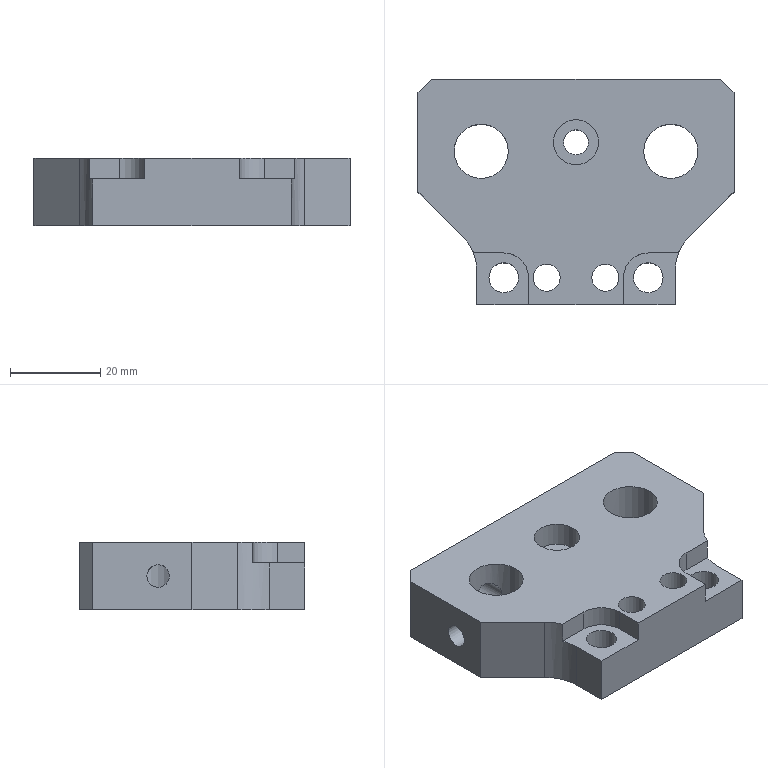Part | NX | features BREP 1 | 1 solid | 34 faces | box 70 x 50 x 15 mm | volume 37859 mm3 | plane 19 | cylinder 15 | commonest cylinder face diameters 5 x3 6 x2 6.6 x2 11 x2 12 x2 20 x2
STEP:
#1=CARTESIAN_POINT('',(35.,22.,0.));
#2=VERTEX_POINT('',#1);
#3=CARTESIAN_POINT('',(32.,25.,0.));
#4=VERTEX_POINT('',#3);
#5=CARTESIAN_POINT('',(35.,22.,0.));
#6=DIRECTION('',(-0.7071,0.7071,0.));
#7=VECTOR('',#6,1000.);
#8=LINE('',#5,#7);
#9=EDGE_CURVE('',#2,#4,#8,.T.);
#10=ORIENTED_EDGE('',*,*,#9,.F.);
#11=CARTESIAN_POINT('',(35.,0.,0.));
#12=VERTEX_POINT('',#11);
#13=CARTESIAN_POINT('',(35.,0.,0.));
#14=DIRECTION('',(0.,1.,0.));
#15=VECTOR('',#14,1000.);
#16=LINE('',#13,#15);
#17=EDGE_CURVE('',#12,#2,#16,.T.);
#18=ORIENTED_EDGE('',*,*,#17,.F.);
#19=CARTESIAN_POINT('',(24.929,-10.071,0.));
#20=VERTEX_POINT('',#19);
#21=CARTESIAN_POINT('',(24.929,-10.071,0.));
#22=DIRECTION('',(0.7071,0.7071,0.));
#23=VECTOR('',#22,1000.);
#24=LINE('',#21,#23);
#25=EDGE_CURVE('',#20,#12,#24,.T.);
#26=ORIENTED_EDGE('',*,*,#25,.F.);
#27=CARTESIAN_POINT('',(22.,-17.142,0.));
#28=VERTEX_POINT('',#27);
#29=CARTESIAN_POINT('',(32.,-17.142,0.));
#30=DIRECTION('',(0.,0.,-1.));
#31=DIRECTION('',(1.,0.,0.));
#32=AXIS2_PLACEMENT_3D('',#29,#30,#31);
#33=CIRCLE('',#32,10.);
#34=EDGE_CURVE('',#28,#20,#33,.T.);
#35=ORIENTED_EDGE('',*,*,#34,.F.);
#36=CARTESIAN_POINT('',(22.,-25.,0.));
#37=VERTEX_POINT('',#36);
#38=CARTESIAN_POINT('',(22.,0.,0.));
#39=DIRECTION('',(0.,1.,0.));
#40=VECTOR('',#39,1000.);
#41=LINE('',#38,#40);
#42=EDGE_CURVE('',#37,#28,#41,.T.);
#43=ORIENTED_EDGE('',*,*,#42,.F.);
#44=CARTESIAN_POINT('',(-22.,-25.,0.));
#45=VERTEX_POINT('',#44);
#46=CARTESIAN_POINT('',(0.,-25.,0.));
#47=DIRECTION('',(1.,0.,0.));
#48=VECTOR('',#47,1000.);
#49=LINE('',#46,#48);
#50=EDGE_CURVE('',#45,#37,#49,.T.);
#51=ORIENTED_EDGE('',*,*,#50,.F.);
#52=CARTESIAN_POINT('',(-22.,-17.142,0.));
#53=VERTEX_POINT('',#52);
#54=CARTESIAN_POINT('',(-22.,0.,0.));
#55=DIRECTION('',(0.,-1.,0.));
#56=VECTOR('',#55,1000.);
#57=LINE('',#54,#56);
#58=EDGE_CURVE('',#53,#45,#57,.T.);
#59=ORIENTED_EDGE('',*,*,#58,.F.);
#60=CARTESIAN_POINT('',(-24.929,-10.071,0.));
#61=VERTEX_POINT('',#60);
#62=CARTESIAN_POINT('',(-32.,-17.142,0.));
#63=DIRECTION('',(0.,0.,-1.));
#64=DIRECTION('',(1.,0.,0.));
#65=AXIS2_PLACEMENT_3D('',#62,#63,#64);
#66=CIRCLE('',#65,10.);
#67=EDGE_CURVE('',#61,#53,#66,.T.);
#68=ORIENTED_EDGE('',*,*,#67,.F.);
#69=CARTESIAN_POINT('',(-35.,0.,0.));
#70=VERTEX_POINT('',#69);
#71=CARTESIAN_POINT('',(-35.,0.,0.));
#72=DIRECTION('',(0.7071,-0.7071,0.));
#73=VECTOR('',#72,1000.);
#74=LINE('',#71,#73);
#75=EDGE_CURVE('',#70,#61,#74,.T.);
#76=ORIENTED_EDGE('',*,*,#75,.F.);
#77=CARTESIAN_POINT('',(-35.,22.,0.));
#78=VERTEX_POINT('',#77);
#79=CARTESIAN_POINT('',(-35.,0.,0.));
#80=DIRECTION('',(0.,-1.,0.));
#81=VECTOR('',#80,1000.);
#82=LINE('',#79,#81);
#83=EDGE_CURVE('',#78,#70,#82,.T.);
#84=ORIENTED_EDGE('',*,*,#83,.F.);
#85=CARTESIAN_POINT('',(-32.,25.,0.));
#86=VERTEX_POINT('',#85);
#87=CARTESIAN_POINT('',(-32.,25.,0.));
#88=DIRECTION('',(-0.7071,-0.7071,0.));
#89=VECTOR('',#88,1000.);
#90=LINE('',#87,#89);
#91=EDGE_CURVE('',#86,#78,#90,.T.);
#92=ORIENTED_EDGE('',*,*,#91,.F.);
#93=CARTESIAN_POINT('',(0.,25.,0.));
#94=DIRECTION('',(-1.,0.,0.));
#95=VECTOR('',#94,1000.);
#96=LINE('',#93,#95);
#97=EDGE_CURVE('',#4,#86,#96,.T.);
#98=ORIENTED_EDGE('',*,*,#97,.F.);
#99=EDGE_LOOP('',(#10,#18,#26,#35,#43,#51,#59,#68,#76,#84,#92,#98));
#100=FACE_BOUND('',#99,.T.);
#101=CARTESIAN_POINT('',(-27.,9.,0.));
#102=VERTEX_POINT('',#101);
#103=CARTESIAN_POINT('',(-21.,9.,0.));
#104=DIRECTION('',(0.,0.,-1.));
#105=DIRECTION('',(-1.,0.,0.));
#106=AXIS2_PLACEMENT_3D('',#103,#104,#105);
#107=CIRCLE('',#106,6.);
#108=EDGE_CURVE('',#102,#102,#107,.T.);
#109=ORIENTED_EDGE('',*,*,#108,.F.);
#110=EDGE_LOOP('',(#109));
#111=FACE_BOUND('',#110,.T.);
#112=CARTESIAN_POINT('',(15.,9.,0.));
#113=VERTEX_POINT('',#112);
#114=CARTESIAN_POINT('',(21.,9.,0.));
#115=DIRECTION('',(0.,0.,-1.));
#116=DIRECTION('',(-1.,0.,0.));
#117=AXIS2_PLACEMENT_3D('',#114,#115,#116);
#118=CIRCLE('',#117,6.);
#119=EDGE_CURVE('',#113,#113,#118,.T.);
#120=ORIENTED_EDGE('',*,*,#119,.F.);
#121=EDGE_LOOP('',(#120));
#122=FACE_BOUND('',#121,.T.);
#123=CARTESIAN_POINT('',(2.75,11.,0.));
#124=VERTEX_POINT('',#123);
#125=CARTESIAN_POINT('',(0.,11.,0.));
#126=DIRECTION('',(0.,0.,-1.));
#127=DIRECTION('',(1.,0.,0.));
#128=AXIS2_PLACEMENT_3D('',#125,#126,#127);
#129=CIRCLE('',#128,2.75);
#130=EDGE_CURVE('',#124,#124,#129,.T.);
#131=ORIENTED_EDGE('',*,*,#130,.F.);
#132=EDGE_LOOP('',(#131));
#133=FACE_BOUND('',#132,.T.);
#134=CARTESIAN_POINT('',(9.5,-19.,0.));
#135=VERTEX_POINT('',#134);
#136=CARTESIAN_POINT('',(6.5,-19.,0.));
#137=DIRECTION('',(0.,0.,-1.));
#138=DIRECTION('',(1.,0.,0.));
#139=AXIS2_PLACEMENT_3D('',#136,#137,#138);
#140=CIRCLE('',#139,3.);
#141=EDGE_CURVE('',#135,#135,#140,.T.);
#142=ORIENTED_EDGE('',*,*,#141,.F.);
#143=EDGE_LOOP('',(#142));
#144=FACE_BOUND('',#143,.T.);
#145=CARTESIAN_POINT('',(-3.5,-19.,0.));
#146=VERTEX_POINT('',#145);
#147=CARTESIAN_POINT('',(-6.5,-19.,0.));
#148=DIRECTION('',(0.,0.,-1.));
#149=DIRECTION('',(1.,0.,0.));
#150=AXIS2_PLACEMENT_3D('',#147,#148,#149);
#151=CIRCLE('',#150,3.);
#152=EDGE_CURVE('',#146,#146,#151,.T.);
#153=ORIENTED_EDGE('',*,*,#152,.F.);
#154=EDGE_LOOP('',(#153));
#155=FACE_BOUND('',#154,.T.);
#156=CARTESIAN_POINT('',(-12.7,-19.,0.));
#157=VERTEX_POINT('',#156);
#158=CARTESIAN_POINT('',(-16.,-19.,0.));
#159=DIRECTION('',(0.,0.,-1.));
#160=DIRECTION('',(1.,0.,0.));
#161=AXIS2_PLACEMENT_3D('',#158,#159,#160);
#162=CIRCLE('',#161,3.3);
#163=EDGE_CURVE('',#157,#157,#162,.T.);
#164=ORIENTED_EDGE('',*,*,#163,.F.);
#165=EDGE_LOOP('',(#164));
#166=FACE_BOUND('',#165,.T.);
#167=CARTESIAN_POINT('',(19.3,-19.,0.));
#168=VERTEX_POINT('',#167);
#169=CARTESIAN_POINT('',(16.,-19.,0.));
#170=DIRECTION('',(0.,0.,-1.));
#171=DIRECTION('',(1.,0.,0.));
#172=AXIS2_PLACEMENT_3D('',#169,#170,#171);
#173=CIRCLE('',#172,3.3);
#174=EDGE_CURVE('',#168,#168,#173,.T.);
#175=ORIENTED_EDGE('',*,*,#174,.F.);
#176=EDGE_LOOP('',(#175));
#177=FACE_BOUND('',#176,.T.);
#178=CARTESIAN_POINT('',(0.,0.,0.));
#179=DIRECTION('',(0.,0.,1.));
#180=DIRECTION('',(-1.,0.,0.));
#181=AXIS2_PLACEMENT_3D('',#178,#179,#180);
#182=PLANE('',#181);
#183=ADVANCED_FACE('',(#100,#111,#122,#133,#144,#155,#166,#177),#182,.F.);
#184=CARTESIAN_POINT('',(32.,25.,15.));
#185=VERTEX_POINT('',#184);
#186=CARTESIAN_POINT('',(32.,25.,15.));
#187=DIRECTION('',(0.,0.,1.));
#188=VECTOR('',#187,1000.);
#189=LINE('',#186,#188);
#190=EDGE_CURVE('',#4,#185,#189,.T.);
#191=ORIENTED_EDGE('',*,*,#190,.F.);
#192=ORIENTED_EDGE('',*,*,#97,.T.);
#193=CARTESIAN_POINT('',(-32.,25.,15.));
#194=VERTEX_POINT('',#193);
#195=CARTESIAN_POINT('',(-32.,25.,15.));
#196=DIRECTION('',(0.,0.,-1.));
#197=VECTOR('',#196,1000.);
#198=LINE('',#195,#197);
#199=EDGE_CURVE('',#194,#86,#198,.T.);
#200=ORIENTED_EDGE('',*,*,#199,.F.);
#201=CARTESIAN_POINT('',(-35.,25.,15.));
#202=DIRECTION('',(-1.,0.,0.));
#203=VECTOR('',#202,1000.);
#204=LINE('',#201,#203);
#205=EDGE_CURVE('',#185,#194,#204,.T.);
#206=ORIENTED_EDGE('',*,*,#205,.F.);
#207=EDGE_LOOP('',(#191,#192,#200,#206));
#208=FACE_BOUND('',#207,.T.);
#209=CARTESIAN_POINT('',(-18.5,25.,10.));
#210=VERTEX_POINT('',#209);
#211=CARTESIAN_POINT('',(-18.5,25.,7.5));
#212=DIRECTION('',(0.,1.,0.));
#213=DIRECTION('',(0.,0.,1.));
#214=AXIS2_PLACEMENT_3D('',#211,#212,#213);
#215=CIRCLE('',#214,2.5);
#216=EDGE_CURVE('',#210,#210,#215,.T.);
#217=ORIENTED_EDGE('',*,*,#216,.F.);
#218=EDGE_LOOP('',(#217));
#219=FACE_BOUND('',#218,.T.);
#220=CARTESIAN_POINT('',(18.5,25.,10.));
#221=VERTEX_POINT('',#220);
#222=CARTESIAN_POINT('',(18.5,25.,7.5));
#223=DIRECTION('',(0.,1.,0.));
#224=DIRECTION('',(0.,0.,1.));
#225=AXIS2_PLACEMENT_3D('',#222,#223,#224);
#226=CIRCLE('',#225,2.5);
#227=EDGE_CURVE('',#221,#221,#226,.T.);
#228=ORIENTED_EDGE('',*,*,#227,.F.);
#229=EDGE_LOOP('',(#228));
#230=FACE_BOUND('',#229,.T.);
#231=CARTESIAN_POINT('',(-35.,25.,15.));
#232=DIRECTION('',(0.,-1.,0.));
#233=DIRECTION('',(0.,0.,1.));
#234=AXIS2_PLACEMENT_3D('',#231,#232,#233);
#235=PLANE('',#234);
#236=ADVANCED_FACE('',(#208,#219,#230),#235,.F.);
#237=CARTESIAN_POINT('',(35.,22.,15.));
#238=VERTEX_POINT('',#237);
#239=CARTESIAN_POINT('',(35.,22.,15.));
#240=DIRECTION('',(0.,0.,1.));
#241=VECTOR('',#240,1000.);
#242=LINE('',#239,#241);
#243=EDGE_CURVE('',#2,#238,#242,.T.);
#244=ORIENTED_EDGE('',*,*,#243,.F.);
#245=ORIENTED_EDGE('',*,*,#9,.T.);
#246=ORIENTED_EDGE('',*,*,#190,.T.);
#247=CARTESIAN_POINT('',(32.,25.,15.));
#248=DIRECTION('',(-0.7071,0.7071,0.));
#249=VECTOR('',#248,1000.);
#250=LINE('',#247,#249);
#251=EDGE_CURVE('',#238,#185,#250,.T.);
#252=ORIENTED_EDGE('',*,*,#251,.F.);
#253=EDGE_LOOP('',(#244,#245,#246,#252));
#254=FACE_BOUND('',#253,.T.);
#255=CARTESIAN_POINT('',(32.,25.,15.));
#256=DIRECTION('',(-0.7071,-0.7071,0.));
#257=DIRECTION('',(-0.7071,0.7071,0.));
#258=AXIS2_PLACEMENT_3D('',#255,#256,#257);
#259=PLANE('',#258);
#260=ADVANCED_FACE('',(#254),#259,.F.);
#261=ORIENTED_EDGE('',*,*,#243,.T.);
#262=CARTESIAN_POINT('',(35.,0.,15.));
#263=VERTEX_POINT('',#262);
#264=CARTESIAN_POINT('',(35.,25.,15.));
#265=DIRECTION('',(0.,1.,0.));
#266=VECTOR('',#265,1000.);
#267=LINE('',#264,#266);
#268=EDGE_CURVE('',#263,#238,#267,.T.);
#269=ORIENTED_EDGE('',*,*,#268,.F.);
#270=CARTESIAN_POINT('',(35.,0.,15.));
#271=DIRECTION('',(0.,0.,1.));
#272=VECTOR('',#271,1000.);
#273=LINE('',#270,#272);
#274=EDGE_CURVE('',#12,#263,#273,.T.);
#275=ORIENTED_EDGE('',*,*,#274,.F.);
#276=ORIENTED_EDGE('',*,*,#17,.T.);
#277=EDGE_LOOP('',(#261,#269,#275,#276));
#278=FACE_BOUND('',#277,.T.);
#279=CARTESIAN_POINT('',(35.,25.,15.));
#280=DIRECTION('',(-1.,0.,0.));
#281=DIRECTION('',(0.,1.,0.));
#282=AXIS2_PLACEMENT_3D('',#279,#280,#281);
#283=PLANE('',#282);
#284=ADVANCED_FACE('',(#278),#283,.F.);
#285=CARTESIAN_POINT('',(24.929,-10.071,15.));
#286=VERTEX_POINT('',#285);
#287=CARTESIAN_POINT('',(24.929,-10.071,15.));
#288=DIRECTION('',(0.,0.,1.));
#289=VECTOR('',#288,1000.);
#290=LINE('',#287,#289);
#291=EDGE_CURVE('',#20,#286,#290,.T.);
#292=ORIENTED_EDGE('',*,*,#291,.F.);
#293=ORIENTED_EDGE('',*,*,#25,.T.);
#294=ORIENTED_EDGE('',*,*,#274,.T.);
#295=CARTESIAN_POINT('',(22.,-13.,15.));
#296=DIRECTION('',(0.7071,0.7071,0.));
#297=VECTOR('',#296,1000.);
#298=LINE('',#295,#297);
#299=EDGE_CURVE('',#286,#263,#298,.T.);
#300=ORIENTED_EDGE('',*,*,#299,.F.);
#301=EDGE_LOOP('',(#292,#293,#294,#300));
#302=FACE_BOUND('',#301,.T.);
#303=CARTESIAN_POINT('',(22.,-13.,15.));
#304=DIRECTION('',(-0.7071,0.7071,0.));
#305=DIRECTION('',(0.7071,0.7071,0.));
#306=AXIS2_PLACEMENT_3D('',#303,#304,#305);
#307=PLANE('',#306);
#308=ADVANCED_FACE('',(#302),#307,.F.);
#309=CARTESIAN_POINT('',(22.,-17.142,10.4));
#310=VERTEX_POINT('',#309);
#311=CARTESIAN_POINT('',(22.687,-13.5,10.4));
#312=VERTEX_POINT('',#311);
#313=CARTESIAN_POINT('',(32.,-17.142,10.4));
#314=DIRECTION('',(0.,0.,-1.));
#315=DIRECTION('',(1.,0.,0.));
#316=AXIS2_PLACEMENT_3D('',#313,#314,#315);
#317=CIRCLE('',#316,10.);
#318=EDGE_CURVE('',#310,#312,#317,.T.);
#319=ORIENTED_EDGE('',*,*,#318,.F.);
#320=CARTESIAN_POINT('',(22.,-17.142,15.));
#321=DIRECTION('',(0.,0.,1.));
#322=VECTOR('',#321,1000.);
#323=LINE('',#320,#322);
#324=EDGE_CURVE('',#28,#310,#323,.T.);
#325=ORIENTED_EDGE('',*,*,#324,.F.);
#326=ORIENTED_EDGE('',*,*,#34,.T.);
#327=ORIENTED_EDGE('',*,*,#291,.T.);
#328=CARTESIAN_POINT('',(22.687,-13.5,15.));
#329=VERTEX_POINT('',#328);
#330=CARTESIAN_POINT('',(32.,-17.142,15.));
#331=DIRECTION('',(0.,0.,-1.));
#332=DIRECTION('',(1.,0.,0.));
#333=AXIS2_PLACEMENT_3D('',#330,#331,#332);
#334=CIRCLE('',#333,10.);
#335=EDGE_CURVE('',#329,#286,#334,.T.);
#336=ORIENTED_EDGE('',*,*,#335,.F.);
#337=CARTESIAN_POINT('',(22.687,-13.5,15.));
#338=DIRECTION('',(0.,0.,1.));
#339=VECTOR('',#338,1000.);
#340=LINE('',#337,#339);
#341=EDGE_CURVE('',#312,#329,#340,.T.);
#342=ORIENTED_EDGE('',*,*,#341,.F.);
#343=EDGE_LOOP('',(#319,#325,#326,#327,#336,#342));
#344=FACE_BOUND('',#343,.T.);
#345=CARTESIAN_POINT('',(32.,-17.142,15.));
#346=DIRECTION('',(0.,0.,1.));
#347=DIRECTION('',(-1.,0.,0.));
#348=AXIS2_PLACEMENT_3D('',#345,#346,#347);
#349=CYLINDRICAL_SURFACE('',#348,10.);
#350=ADVANCED_FACE('',(#344),#349,.F.);
#351=CARTESIAN_POINT('',(22.,-25.,10.4));
#352=VERTEX_POINT('',#351);
#353=CARTESIAN_POINT('',(22.,-25.,10.4));
#354=DIRECTION('',(0.,1.,0.));
#355=VECTOR('',#354,1000.);
#356=LINE('',#353,#355);
#357=EDGE_CURVE('',#352,#310,#356,.T.);
#358=ORIENTED_EDGE('',*,*,#357,.F.);
#359=CARTESIAN_POINT('',(22.,-25.,15.));
#360=DIRECTION('',(0.,0.,1.));
#361=VECTOR('',#360,1000.);
#362=LINE('',#359,#361);
#363=EDGE_CURVE('',#37,#352,#362,.T.);
#364=ORIENTED_EDGE('',*,*,#363,.F.);
#365=ORIENTED_EDGE('',*,*,#42,.T.);
#366=ORIENTED_EDGE('',*,*,#324,.T.);
#367=EDGE_LOOP('',(#358,#364,#365,#366));
#368=FACE_BOUND('',#367,.T.);
#369=CARTESIAN_POINT('',(22.,-25.,15.));
#370=DIRECTION('',(-1.,0.,0.));
#371=DIRECTION('',(0.,0.,-1.));
#372=AXIS2_PLACEMENT_3D('',#369,#370,#371);
#373=PLANE('',#372);
#374=ADVANCED_FACE('',(#368),#373,.F.);
#375=CARTESIAN_POINT('',(-22.,-25.,10.4));
#376=VERTEX_POINT('',#375);
#377=CARTESIAN_POINT('',(-10.5,-25.,10.4));
#378=VERTEX_POINT('',#377);
#379=CARTESIAN_POINT('',(-35.,-25.,10.4));
#380=DIRECTION('',(1.,0.,0.));
#381=VECTOR('',#380,1000.);
#382=LINE('',#379,#381);
#383=EDGE_CURVE('',#376,#378,#382,.T.);
#384=ORIENTED_EDGE('',*,*,#383,.F.);
#385=CARTESIAN_POINT('',(-22.,-25.,15.));
#386=DIRECTION('',(0.,0.,1.));
#387=VECTOR('',#386,1000.);
#388=LINE('',#385,#387);
#389=EDGE_CURVE('',#45,#376,#388,.T.);
#390=ORIENTED_EDGE('',*,*,#389,.F.);
#391=ORIENTED_EDGE('',*,*,#50,.T.);
#392=ORIENTED_EDGE('',*,*,#363,.T.);
#393=CARTESIAN_POINT('',(10.5,-25.,10.4));
#394=VERTEX_POINT('',#393);
#395=CARTESIAN_POINT('',(-35.,-25.,10.4));
#396=DIRECTION('',(1.,0.,0.));
#397=VECTOR('',#396,1000.);
#398=LINE('',#395,#397);
#399=EDGE_CURVE('',#394,#352,#398,.T.);
#400=ORIENTED_EDGE('',*,*,#399,.F.);
#401=CARTESIAN_POINT('',(10.5,-25.,15.));
#402=VERTEX_POINT('',#401);
#403=CARTESIAN_POINT('',(10.5,-25.,15.));
#404=DIRECTION('',(0.,0.,-1.));
#405=VECTOR('',#404,1000.);
#406=LINE('',#403,#405);
#407=EDGE_CURVE('',#402,#394,#406,.T.);
#408=ORIENTED_EDGE('',*,*,#407,.F.);
#409=CARTESIAN_POINT('',(-10.5,-25.,15.));
#410=VERTEX_POINT('',#409);
#411=CARTESIAN_POINT('',(-35.,-25.,15.));
#412=DIRECTION('',(1.,0.,0.));
#413=VECTOR('',#412,1000.);
#414=LINE('',#411,#413);
#415=EDGE_CURVE('',#410,#402,#414,.T.);
#416=ORIENTED_EDGE('',*,*,#415,.F.);
#417=CARTESIAN_POINT('',(-10.5,-25.,15.));
#418=DIRECTION('',(0.,0.,1.));
#419=VECTOR('',#418,1000.);
#420=LINE('',#417,#419);
#421=EDGE_CURVE('',#378,#410,#420,.T.);
#422=ORIENTED_EDGE('',*,*,#421,.F.);
#423=EDGE_LOOP('',(#384,#390,#391,#392,#400,#408,#416,#422));
#424=FACE_BOUND('',#423,.T.);
#425=CARTESIAN_POINT('',(-35.,-25.,15.));
#426=DIRECTION('',(0.,1.,0.));
#427=DIRECTION('',(0.,0.,-1.));
#428=AXIS2_PLACEMENT_3D('',#425,#426,#427);
#429=PLANE('',#428);
#430=ADVANCED_FACE('',(#424),#429,.F.);
#431=ORIENTED_EDGE('',*,*,#58,.T.);
#432=ORIENTED_EDGE('',*,*,#389,.T.);
#433=CARTESIAN_POINT('',(-22.,-17.142,10.4));
#434=VERTEX_POINT('',#433);
#435=CARTESIAN_POINT('',(-22.,-25.,10.4));
#436=DIRECTION('',(0.,1.,0.));
#437=VECTOR('',#436,1000.);
#438=LINE('',#435,#437);
#439=EDGE_CURVE('',#376,#434,#438,.T.);
#440=ORIENTED_EDGE('',*,*,#439,.T.);
#441=CARTESIAN_POINT('',(-22.,-17.142,15.));
#442=DIRECTION('',(0.,0.,-1.));
#443=VECTOR('',#442,1000.);
#444=LINE('',#441,#443);
#445=EDGE_CURVE('',#434,#53,#444,.T.);
#446=ORIENTED_EDGE('',*,*,#445,.T.);
#447=EDGE_LOOP('',(#431,#432,#440,#446));
#448=FACE_BOUND('',#447,.T.);
#449=CARTESIAN_POINT('',(-22.,-25.,15.));
#450=DIRECTION('',(-1.,0.,0.));
#451=DIRECTION('',(0.,0.,-1.));
#452=AXIS2_PLACEMENT_3D('',#449,#450,#451);
#453=PLANE('',#452);
#454=ADVANCED_FACE('',(#448),#453,.T.);
#455=CARTESIAN_POINT('',(-24.929,-10.071,15.));
#456=VERTEX_POINT('',#455);
#457=CARTESIAN_POINT('',(-22.687,-13.5,15.));
#458=VERTEX_POINT('',#457);
#459=CARTESIAN_POINT('',(-32.,-17.142,15.));
#460=DIRECTION('',(0.,0.,-1.));
#461=DIRECTION('',(1.,0.,0.));
#462=AXIS2_PLACEMENT_3D('',#459,#460,#461);
#463=CIRCLE('',#462,10.);
#464=EDGE_CURVE('',#456,#458,#463,.T.);
#465=ORIENTED_EDGE('',*,*,#464,.F.);
#466=CARTESIAN_POINT('',(-24.929,-10.071,15.));
#467=DIRECTION('',(0.,0.,1.));
#468=VECTOR('',#467,1000.);
#469=LINE('',#466,#468);
#470=EDGE_CURVE('',#61,#456,#469,.T.);
#471=ORIENTED_EDGE('',*,*,#470,.F.);
#472=ORIENTED_EDGE('',*,*,#67,.T.);
#473=ORIENTED_EDGE('',*,*,#445,.F.);
#474=CARTESIAN_POINT('',(-22.687,-13.5,10.4));
#475=VERTEX_POINT('',#474);
#476=CARTESIAN_POINT('',(-32.,-17.142,10.4));
#477=DIRECTION('',(0.,0.,-1.));
#478=DIRECTION('',(1.,0.,0.));
#479=AXIS2_PLACEMENT_3D('',#476,#477,#478);
#480=CIRCLE('',#479,10.);
#481=EDGE_CURVE('',#475,#434,#480,.T.);
#482=ORIENTED_EDGE('',*,*,#481,.F.);
#483=CARTESIAN_POINT('',(-22.687,-13.5,15.));
#484=DIRECTION('',(0.,0.,-1.));
#485=VECTOR('',#484,1000.);
#486=LINE('',#483,#485);
#487=EDGE_CURVE('',#458,#475,#486,.T.);
#488=ORIENTED_EDGE('',*,*,#487,.F.);
#489=EDGE_LOOP('',(#465,#471,#472,#473,#482,#488));
#490=FACE_BOUND('',#489,.T.);
#491=CARTESIAN_POINT('',(-32.,-17.142,15.));
#492=DIRECTION('',(0.,0.,1.));
#493=DIRECTION('',(-1.,0.,0.));
#494=AXIS2_PLACEMENT_3D('',#491,#492,#493);
#495=CYLINDRICAL_SURFACE('',#494,10.);
#496=ADVANCED_FACE('',(#490),#495,.F.);
#497=CARTESIAN_POINT('',(-35.,0.,15.));
#498=VERTEX_POINT('',#497);
#499=CARTESIAN_POINT('',(-22.,-13.,15.));
#500=DIRECTION('',(-0.7071,0.7071,0.));
#501=VECTOR('',#500,1000.);
#502=LINE('',#499,#501);
#503=EDGE_CURVE('',#456,#498,#502,.T.);
#504=ORIENTED_EDGE('',*,*,#503,.T.);
#505=CARTESIAN_POINT('',(-35.,0.,15.));
#506=DIRECTION('',(0.,0.,-1.));
#507=VECTOR('',#506,1000.);
#508=LINE('',#505,#507);
#509=EDGE_CURVE('',#498,#70,#508,.T.);
#510=ORIENTED_EDGE('',*,*,#509,.T.);
#511=ORIENTED_EDGE('',*,*,#75,.T.);
#512=ORIENTED_EDGE('',*,*,#470,.T.);
#513=EDGE_LOOP('',(#504,#510,#511,#512));
#514=FACE_BOUND('',#513,.T.);
#515=CARTESIAN_POINT('',(-22.,-13.,15.));
#516=DIRECTION('',(-0.7071,-0.7071,0.));
#517=DIRECTION('',(-0.7071,0.7071,0.));
#518=AXIS2_PLACEMENT_3D('',#515,#516,#517);
#519=PLANE('',#518);
#520=ADVANCED_FACE('',(#514),#519,.T.);
#521=CARTESIAN_POINT('',(-35.,22.,15.));
#522=VERTEX_POINT('',#521);
#523=CARTESIAN_POINT('',(-35.,22.,15.));
#524=DIRECTION('',(0.,0.,1.));
#525=VECTOR('',#524,1000.);
#526=LINE('',#523,#525);
#527=EDGE_CURVE('',#78,#522,#526,.T.);
#528=ORIENTED_EDGE('',*,*,#527,.F.);
#529=ORIENTED_EDGE('',*,*,#83,.T.);
#530=ORIENTED_EDGE('',*,*,#509,.F.);
#531=CARTESIAN_POINT('',(-35.,25.,15.));
#532=DIRECTION('',(0.,-1.,0.));
#533=VECTOR('',#532,1000.);
#534=LINE('',#531,#533);
#535=EDGE_CURVE('',#522,#498,#534,.T.);
#536=ORIENTED_EDGE('',*,*,#535,.F.);
#537=EDGE_LOOP('',(#528,#529,#530,#536));
#538=FACE_BOUND('',#537,.T.);
#539=CARTESIAN_POINT('',(-35.,7.5,10.));
#540=VERTEX_POINT('',#539);
#541=CARTESIAN_POINT('',(-35.,7.5,7.5));
#542=DIRECTION('',(-1.,0.,0.));
#543=DIRECTION('',(0.,0.,1.));
#544=AXIS2_PLACEMENT_3D('',#541,#542,#543);
#545=CIRCLE('',#544,2.5);
#546=EDGE_CURVE('',#540,#540,#545,.T.);
#547=ORIENTED_EDGE('',*,*,#546,.F.);
#548=EDGE_LOOP('',(#547));
#549=FACE_BOUND('',#548,.T.);
#550=CARTESIAN_POINT('',(-35.,25.,15.));
#551=DIRECTION('',(1.,0.,0.));
#552=DIRECTION('',(0.,-1.,0.));
#553=AXIS2_PLACEMENT_3D('',#550,#551,#552);
#554=PLANE('',#553);
#555=ADVANCED_FACE('',(#538,#549),#554,.F.);
#556=ORIENTED_EDGE('',*,*,#199,.T.);
#557=ORIENTED_EDGE('',*,*,#91,.T.);
#558=ORIENTED_EDGE('',*,*,#527,.T.);
#559=CARTESIAN_POINT('',(-35.,22.,15.));
#560=DIRECTION('',(-0.7071,-0.7071,0.));
#561=VECTOR('',#560,1000.);
#562=LINE('',#559,#561);
#563=EDGE_CURVE('',#194,#522,#562,.T.);
#564=ORIENTED_EDGE('',*,*,#563,.F.);
#565=EDGE_LOOP('',(#556,#557,#558,#564));
#566=FACE_BOUND('',#565,.T.);
#567=CARTESIAN_POINT('',(-35.,22.,15.));
#568=DIRECTION('',(0.7071,-0.7071,0.));
#569=DIRECTION('',(-0.7071,-0.7071,0.));
#570=AXIS2_PLACEMENT_3D('',#567,#568,#569);
#571=PLANE('',#570);
#572=ADVANCED_FACE('',(#566),#571,.F.);
#573=CARTESIAN_POINT('',(-27.,9.,5.5));
#574=VERTEX_POINT('',#573);
#575=CARTESIAN_POINT('',(-26.807,7.03,4.78));
#576=CARTESIAN_POINT('',(-27.085,9.176,5.261));
#577=CARTESIAN_POINT('',(-26.853,10.268,7.177));
#578=CARTESIAN_POINT('',(-27.018,9.651,9.286));
#579=CARTESIAN_POINT('',(-26.986,7.66,10.271));
#580=CARTESIAN_POINT('',(-26.287,6.069,9.706));
#581=CARTESIAN_POINT('',(-25.715,5.274,8.763));
#582=CARTESIAN_POINT('',(-25.424,4.947,7.808));
#583=CARTESIAN_POINT('',(-25.513,5.042,6.762));
#584=CARTESIAN_POINT('',(-26.015,5.648,5.63));
#585=CARTESIAN_POINT('',(-26.807,7.03,4.78));
#586=CARTESIAN_POINT('',(-27.085,9.176,5.261));
#587=CARTESIAN_POINT('',(-26.853,10.268,7.177));
#588=B_SPLINE_CURVE_WITH_KNOTS('',3,(#575,#576,#577,#578,#579,#580,#581,#582,#583,#584,#585,#586,#587),.UNSPECIFIED.,.T.,.F.,(1,1,1,1,1,1,1,1,1,1,1,1,1,1,1,1,1),(-0.005047,-0.004037,-0.002019,0.,0.002019,0.004037,0.006056,0.008075,0.009084,0.01009,0.0111,0.01211,0.01413,0.01615,0.01817,0.02019,0.02221),.UNSPECIFIED.);
#589=EDGE_CURVE('',#574,#574,#588,.T.);
#590=ORIENTED_EDGE('',*,*,#589,.F.);
#591=EDGE_LOOP('',(#590));
#592=FACE_BOUND('',#591,.T.);
#593=CARTESIAN_POINT('',(-27.,9.,15.));
#594=VERTEX_POINT('',#593);
#595=CARTESIAN_POINT('',(-21.,9.,15.));
#596=DIRECTION('',(0.,0.,-1.));
#597=DIRECTION('',(-1.,0.,0.));
#598=AXIS2_PLACEMENT_3D('',#595,#596,#597);
#599=CIRCLE('',#598,6.);
#600=EDGE_CURVE('',#594,#594,#599,.T.);
#601=ORIENTED_EDGE('',*,*,#600,.F.);
#602=EDGE_LOOP('',(#601));
#603=FACE_BOUND('',#602,.T.);
#604=CARTESIAN_POINT('',(-18.5,14.454,5.));
#605=VERTEX_POINT('',#604);
#606=CARTESIAN_POINT('',(-20.564,15.052,5.57));
#607=CARTESIAN_POINT('',(-18.791,14.667,4.867));
#608=CARTESIAN_POINT('',(-17.564,13.953,5.126));
#609=CARTESIAN_POINT('',(-16.814,13.331,5.59));
#610=CARTESIAN_POINT('',(-16.268,12.714,6.256));
#611=CARTESIAN_POINT('',(-15.936,12.22,7.216));
#612=CARTESIAN_POINT('',(-16.067,12.428,8.324));
#613=CARTESIAN_POINT('',(-16.524,13.027,9.108));
#614=CARTESIAN_POINT('',(-17.173,13.652,9.676));
#615=CARTESIAN_POINT('',(-18.287,14.44,10.128));
#616=CARTESIAN_POINT('',(-20.104,15.034,9.816));
#617=CARTESIAN_POINT('',(-21.312,14.978,7.798));
#618=CARTESIAN_POINT('',(-20.564,15.052,5.57));
#619=CARTESIAN_POINT('',(-18.791,14.667,4.867));
#620=CARTESIAN_POINT('',(-17.564,13.953,5.126));
#621=B_SPLINE_CURVE_WITH_KNOTS('',3,(#606,#607,#608,#609,#610,#611,#612,#613,#614,#615,#616,#617,#618,#619,#620),.UNSPECIFIED.,.T.,.F.,(1,1,1,1,1,1,1,1,1,1,1,1,1,1,1,1,1,1,1),(-0.006348,-0.004232,-0.002116,0.,0.001058,0.002116,0.003174,0.004232,0.00529,0.006348,0.007406,0.008464,0.01058,0.0127,0.01481,0.01693,0.01799,0.01904,0.0201),.UNSPECIFIED.);
#622=EDGE_CURVE('',#605,#605,#621,.T.);
#623=ORIENTED_EDGE('',*,*,#622,.F.);
#624=EDGE_LOOP('',(#623));
#625=FACE_BOUND('',#624,.T.);
#626=ORIENTED_EDGE('',*,*,#108,.T.);
#627=EDGE_LOOP('',(#626));
#628=FACE_BOUND('',#627,.T.);
#629=CARTESIAN_POINT('',(-21.,9.,0.));
#630=DIRECTION('',(0.,0.,-1.));
#631=DIRECTION('',(1.,0.,0.));
#632=AXIS2_PLACEMENT_3D('',#629,#630,#631);
#633=CYLINDRICAL_SURFACE('',#632,6.);
#634=ADVANCED_FACE('',(#592,#603,#625,#628),#633,.F.);
#635=CARTESIAN_POINT('',(15.,9.,15.));
#636=VERTEX_POINT('',#635);
#637=CARTESIAN_POINT('',(21.,9.,15.));
#638=DIRECTION('',(0.,0.,-1.));
#639=DIRECTION('',(-1.,0.,0.));
#640=AXIS2_PLACEMENT_3D('',#637,#638,#639);
#641=CIRCLE('',#640,6.);
#642=EDGE_CURVE('',#636,#636,#641,.T.);
#643=ORIENTED_EDGE('',*,*,#642,.F.);
#644=EDGE_LOOP('',(#643));
#645=FACE_BOUND('',#644,.T.);
#646=CARTESIAN_POINT('',(18.5,14.454,5.));
#647=VERTEX_POINT('',#646);
#648=CARTESIAN_POINT('',(17.561,13.951,5.127));
#649=CARTESIAN_POINT('',(18.793,14.668,4.866));
#650=CARTESIAN_POINT('',(20.559,15.052,5.568));
#651=CARTESIAN_POINT('',(21.312,14.978,7.792));
#652=CARTESIAN_POINT('',(20.113,15.035,9.81));
#653=CARTESIAN_POINT('',(18.294,14.444,10.129));
#654=CARTESIAN_POINT('',(17.177,13.656,9.679));
#655=CARTESIAN_POINT('',(16.525,13.028,9.109));
#656=CARTESIAN_POINT('',(16.069,12.431,8.33));
#657=CARTESIAN_POINT('',(15.936,12.219,7.221));
#658=CARTESIAN_POINT('',(16.265,12.711,6.261));
#659=CARTESIAN_POINT('',(16.815,13.331,5.589));
#660=CARTESIAN_POINT('',(17.561,13.951,5.127));
#661=CARTESIAN_POINT('',(18.793,14.668,4.866));
#662=CARTESIAN_POINT('',(20.559,15.052,5.568));
#663=B_SPLINE_CURVE_WITH_KNOTS('',3,(#648,#649,#650,#651,#652,#653,#654,#655,#656,#657,#658,#659,#660,#661,#662),.UNSPECIFIED.,.T.,.F.,(1,1,1,1,1,1,1,1,1,1,1,1,1,1,1,1,1,1,1),(-0.00318,-0.00212,-0.00106,0.,0.00212,0.004239,0.006359,0.008479,0.009539,0.0106,0.01166,0.01272,0.01378,0.01484,0.0159,0.01696,0.01908,0.0212,0.02332),.UNSPECIFIED.);
#664=EDGE_CURVE('',#647,#647,#663,.T.);
#665=ORIENTED_EDGE('',*,*,#664,.F.);
#666=EDGE_LOOP('',(#665));
#667=FACE_BOUND('',#666,.T.);
#668=ORIENTED_EDGE('',*,*,#119,.T.);
#669=EDGE_LOOP('',(#668));
#670=FACE_BOUND('',#669,.T.);
#671=CARTESIAN_POINT('',(21.,9.,0.));
#672=DIRECTION('',(0.,0.,-1.));
#673=DIRECTION('',(1.,0.,0.));
#674=AXIS2_PLACEMENT_3D('',#671,#672,#673);
#675=CYLINDRICAL_SURFACE('',#674,6.);
#676=ADVANCED_FACE('',(#645,#667,#670),#675,.F.);
#677=ORIENTED_EDGE('',*,*,#130,.T.);
#678=EDGE_LOOP('',(#677));
#679=FACE_BOUND('',#678,.T.);
#680=CARTESIAN_POINT('',(2.75,11.,9.6));
#681=VERTEX_POINT('',#680);
#682=CARTESIAN_POINT('',(0.,11.,9.6));
#683=DIRECTION('',(0.,0.,-1.));
#684=DIRECTION('',(1.,0.,0.));
#685=AXIS2_PLACEMENT_3D('',#682,#683,#684);
#686=CIRCLE('',#685,2.75);
#687=EDGE_CURVE('',#681,#681,#686,.T.);
#688=ORIENTED_EDGE('',*,*,#687,.F.);
#689=EDGE_LOOP('',(#688));
#690=FACE_BOUND('',#689,.T.);
#691=CARTESIAN_POINT('',(0.,11.,15.));
#692=DIRECTION('',(0.,0.,1.));
#693=DIRECTION('',(-1.,0.,0.));
#694=AXIS2_PLACEMENT_3D('',#691,#692,#693);
#695=CYLINDRICAL_SURFACE('',#694,2.75);
#696=ADVANCED_FACE('',(#679,#690),#695,.F.);
#697=ORIENTED_EDGE('',*,*,#141,.T.);
#698=EDGE_LOOP('',(#697));
#699=FACE_BOUND('',#698,.T.);
#700=CARTESIAN_POINT('',(9.5,-19.,15.));
#701=VERTEX_POINT('',#700);
#702=CARTESIAN_POINT('',(6.5,-19.,15.));
#703=DIRECTION('',(0.,0.,-1.));
#704=DIRECTION('',(1.,0.,0.));
#705=AXIS2_PLACEMENT_3D('',#702,#703,#704);
#706=CIRCLE('',#705,3.);
#707=EDGE_CURVE('',#701,#701,#706,.T.);
#708=ORIENTED_EDGE('',*,*,#707,.F.);
#709=EDGE_LOOP('',(#708));
#710=FACE_BOUND('',#709,.T.);
#711=CARTESIAN_POINT('',(6.5,-19.,15.));
#712=DIRECTION('',(0.,0.,1.));
#713=DIRECTION('',(-1.,0.,0.));
#714=AXIS2_PLACEMENT_3D('',#711,#712,#713);
#715=CYLINDRICAL_SURFACE('',#714,3.);
#716=ADVANCED_FACE('',(#699,#710),#715,.F.);
#717=ORIENTED_EDGE('',*,*,#152,.T.);
#718=EDGE_LOOP('',(#717));
#719=FACE_BOUND('',#718,.T.);
#720=CARTESIAN_POINT('',(-3.5,-19.,15.));
#721=VERTEX_POINT('',#720);
#722=CARTESIAN_POINT('',(-6.5,-19.,15.));
#723=DIRECTION('',(0.,0.,-1.));
#724=DIRECTION('',(1.,0.,0.));
#725=AXIS2_PLACEMENT_3D('',#722,#723,#724);
#726=CIRCLE('',#725,3.);
#727=EDGE_CURVE('',#721,#721,#726,.T.);
#728=ORIENTED_EDGE('',*,*,#727,.F.);
#729=EDGE_LOOP('',(#728));
#730=FACE_BOUND('',#729,.T.);
#731=CARTESIAN_POINT('',(-6.5,-19.,15.));
#732=DIRECTION('',(0.,0.,1.));
#733=DIRECTION('',(-1.,0.,0.));
#734=AXIS2_PLACEMENT_3D('',#731,#732,#733);
#735=CYLINDRICAL_SURFACE('',#734,3.);
#736=ADVANCED_FACE('',(#719,#730),#735,.F.);
#737=ORIENTED_EDGE('',*,*,#163,.T.);
#738=EDGE_LOOP('',(#737));
#739=FACE_BOUND('',#738,.T.);
#740=CARTESIAN_POINT('',(-12.7,-19.,10.4));
#741=VERTEX_POINT('',#740);
#742=CARTESIAN_POINT('',(-16.,-19.,10.4));
#743=DIRECTION('',(0.,0.,-1.));
#744=DIRECTION('',(1.,0.,0.));
#745=AXIS2_PLACEMENT_3D('',#742,#743,#744);
#746=CIRCLE('',#745,3.3);
#747=EDGE_CURVE('',#741,#741,#746,.T.);
#748=ORIENTED_EDGE('',*,*,#747,.F.);
#749=EDGE_LOOP('',(#748));
#750=FACE_BOUND('',#749,.T.);
#751=CARTESIAN_POINT('',(-16.,-19.,15.));
#752=DIRECTION('',(0.,0.,1.));
#753=DIRECTION('',(-1.,0.,0.));
#754=AXIS2_PLACEMENT_3D('',#751,#752,#753);
#755=CYLINDRICAL_SURFACE('',#754,3.3);
#756=ADVANCED_FACE('',(#739,#750),#755,.F.);
#757=ORIENTED_EDGE('',*,*,#174,.T.);
#758=EDGE_LOOP('',(#757));
#759=FACE_BOUND('',#758,.T.);
#760=CARTESIAN_POINT('',(19.3,-19.,10.4));
#761=VERTEX_POINT('',#760);
#762=CARTESIAN_POINT('',(16.,-19.,10.4));
#763=DIRECTION('',(0.,0.,-1.));
#764=DIRECTION('',(1.,0.,0.));
#765=AXIS2_PLACEMENT_3D('',#762,#763,#764);
#766=CIRCLE('',#765,3.3);
#767=EDGE_CURVE('',#761,#761,#766,.T.);
#768=ORIENTED_EDGE('',*,*,#767,.F.);
#769=EDGE_LOOP('',(#768));
#770=FACE_BOUND('',#769,.T.);
#771=CARTESIAN_POINT('',(16.,-19.,15.));
#772=DIRECTION('',(0.,0.,1.));
#773=DIRECTION('',(-1.,0.,0.));
#774=AXIS2_PLACEMENT_3D('',#771,#772,#773);
#775=CYLINDRICAL_SURFACE('',#774,3.3);
#776=ADVANCED_FACE('',(#759,#770),#775,.F.);
#777=ORIENTED_EDGE('',*,*,#535,.T.);
#778=ORIENTED_EDGE('',*,*,#503,.F.);
#779=ORIENTED_EDGE('',*,*,#464,.T.);
#780=CARTESIAN_POINT('',(-16.,-13.5,15.));
#781=VERTEX_POINT('',#780);
#782=CARTESIAN_POINT('',(0.,-13.5,15.));
#783=DIRECTION('',(1.,0.,0.));
#784=VECTOR('',#783,1000.);
#785=LINE('',#782,#784);
#786=EDGE_CURVE('',#458,#781,#785,.T.);
#787=ORIENTED_EDGE('',*,*,#786,.T.);
#788=CARTESIAN_POINT('',(-10.5,-19.,15.));
#789=VERTEX_POINT('',#788);
#790=CARTESIAN_POINT('',(-16.,-19.,15.));
#791=DIRECTION('',(0.,0.,-1.));
#792=DIRECTION('',(1.,0.,0.));
#793=AXIS2_PLACEMENT_3D('',#790,#791,#792);
#794=CIRCLE('',#793,5.5);
#795=EDGE_CURVE('',#781,#789,#794,.T.);
#796=ORIENTED_EDGE('',*,*,#795,.T.);
#797=CARTESIAN_POINT('',(-10.5,0.,15.));
#798=DIRECTION('',(0.,-1.,0.));
#799=VECTOR('',#798,1000.);
#800=LINE('',#797,#799);
#801=EDGE_CURVE('',#789,#410,#800,.T.);
#802=ORIENTED_EDGE('',*,*,#801,.T.);
#803=ORIENTED_EDGE('',*,*,#415,.T.);
#804=CARTESIAN_POINT('',(10.5,-19.,15.));
#805=VERTEX_POINT('',#804);
#806=CARTESIAN_POINT('',(10.5,0.,15.));
#807=DIRECTION('',(0.,1.,0.));
#808=VECTOR('',#807,1000.);
#809=LINE('',#806,#808);
#810=EDGE_CURVE('',#402,#805,#809,.T.);
#811=ORIENTED_EDGE('',*,*,#810,.T.);
#812=CARTESIAN_POINT('',(16.,-13.5,15.));
#813=VERTEX_POINT('',#812);
#814=CARTESIAN_POINT('',(16.,-19.,15.));
#815=DIRECTION('',(0.,0.,-1.));
#816=DIRECTION('',(1.,0.,0.));
#817=AXIS2_PLACEMENT_3D('',#814,#815,#816);
#818=CIRCLE('',#817,5.5);
#819=EDGE_CURVE('',#805,#813,#818,.T.);
#820=ORIENTED_EDGE('',*,*,#819,.T.);
#821=CARTESIAN_POINT('',(0.,-13.5,15.));
#822=DIRECTION('',(1.,0.,0.));
#823=VECTOR('',#822,1000.);
#824=LINE('',#821,#823);
#825=EDGE_CURVE('',#813,#329,#824,.T.);
#826=ORIENTED_EDGE('',*,*,#825,.T.);
#827=ORIENTED_EDGE('',*,*,#335,.T.);
#828=ORIENTED_EDGE('',*,*,#299,.T.);
#829=ORIENTED_EDGE('',*,*,#268,.T.);
#830=ORIENTED_EDGE('',*,*,#251,.T.);
#831=ORIENTED_EDGE('',*,*,#205,.T.);
#832=ORIENTED_EDGE('',*,*,#563,.T.);
#833=EDGE_LOOP('',(#777,#778,#779,#787,#796,#802,#803,#811,#820,#826,#827,#828,#829,#830,#831,#832));
#834=FACE_BOUND('',#833,.T.);
#835=ORIENTED_EDGE('',*,*,#642,.T.);
#836=EDGE_LOOP('',(#835));
#837=FACE_BOUND('',#836,.T.);
#838=ORIENTED_EDGE('',*,*,#600,.T.);
#839=EDGE_LOOP('',(#838));
#840=FACE_BOUND('',#839,.T.);
#841=CARTESIAN_POINT('',(5.,11.,15.));
#842=VERTEX_POINT('',#841);
#843=CARTESIAN_POINT('',(0.,11.,15.));
#844=DIRECTION('',(0.,0.,-1.));
#845=DIRECTION('',(1.,0.,0.));
#846=AXIS2_PLACEMENT_3D('',#843,#844,#845);
#847=CIRCLE('',#846,5.);
#848=EDGE_CURVE('',#842,#842,#847,.T.);
#849=ORIENTED_EDGE('',*,*,#848,.T.);
#850=EDGE_LOOP('',(#849));
#851=FACE_BOUND('',#850,.T.);
#852=ORIENTED_EDGE('',*,*,#707,.T.);
#853=EDGE_LOOP('',(#852));
#854=FACE_BOUND('',#853,.T.);
#855=ORIENTED_EDGE('',*,*,#727,.T.);
#856=EDGE_LOOP('',(#855));
#857=FACE_BOUND('',#856,.T.);
#858=CARTESIAN_POINT('',(0.,0.,15.));
#859=DIRECTION('',(0.,0.,1.));
#860=DIRECTION('',(-1.,0.,0.));
#861=AXIS2_PLACEMENT_3D('',#858,#859,#860);
#862=PLANE('',#861);
#863=ADVANCED_FACE('',(#834,#837,#840,#851,#854,#857),#862,.T.);
#864=ORIENTED_EDGE('',*,*,#622,.T.);
#865=EDGE_LOOP('',(#864));
#866=FACE_BOUND('',#865,.T.);
#867=ORIENTED_EDGE('',*,*,#216,.T.);
#868=EDGE_LOOP('',(#867));
#869=FACE_BOUND('',#868,.T.);
#870=CARTESIAN_POINT('',(-18.5,25.,7.5));
#871=DIRECTION('',(0.,1.,0.));
#872=DIRECTION('',(0.,0.,-1.));
#873=AXIS2_PLACEMENT_3D('',#870,#871,#872);
#874=CYLINDRICAL_SURFACE('',#873,2.5);
#875=ADVANCED_FACE('',(#866,#869),#874,.F.);
#876=ORIENTED_EDGE('',*,*,#664,.T.);
#877=EDGE_LOOP('',(#876));
#878=FACE_BOUND('',#877,.T.);
#879=ORIENTED_EDGE('',*,*,#227,.T.);
#880=EDGE_LOOP('',(#879));
#881=FACE_BOUND('',#880,.T.);
#882=CARTESIAN_POINT('',(18.5,25.,7.5));
#883=DIRECTION('',(0.,1.,0.));
#884=DIRECTION('',(0.,0.,-1.));
#885=AXIS2_PLACEMENT_3D('',#882,#883,#884);
#886=CYLINDRICAL_SURFACE('',#885,2.5);
#887=ADVANCED_FACE('',(#878,#881),#886,.F.);
#888=ORIENTED_EDGE('',*,*,#825,.F.);
#889=CARTESIAN_POINT('',(16.,-13.5,10.4));
#890=VERTEX_POINT('',#889);
#891=CARTESIAN_POINT('',(16.,-13.5,-6.356));
#892=DIRECTION('',(0.,0.,1.));
#893=VECTOR('',#892,1000.);
#894=LINE('',#891,#893);
#895=EDGE_CURVE('',#890,#813,#894,.T.);
#896=ORIENTED_EDGE('',*,*,#895,.F.);
#897=CARTESIAN_POINT('',(16.,-13.5,10.4));
#898=DIRECTION('',(-1.,0.,0.));
#899=VECTOR('',#898,1000.);
#900=LINE('',#897,#899);
#901=EDGE_CURVE('',#312,#890,#900,.T.);
#902=ORIENTED_EDGE('',*,*,#901,.F.);
#903=ORIENTED_EDGE('',*,*,#341,.T.);
#904=EDGE_LOOP('',(#888,#896,#902,#903));
#905=FACE_BOUND('',#904,.T.);
#906=CARTESIAN_POINT('',(16.,-13.5,-6.356));
#907=DIRECTION('',(0.,1.,0.));
#908=DIRECTION('',(0.,0.,-1.));
#909=AXIS2_PLACEMENT_3D('',#906,#907,#908);
#910=PLANE('',#909);
#911=ADVANCED_FACE('',(#905),#910,.F.);
#912=ORIENTED_EDGE('',*,*,#767,.T.);
#913=EDGE_LOOP('',(#912));
#914=FACE_BOUND('',#913,.T.);
#915=CARTESIAN_POINT('',(10.5,-19.,10.4));
#916=VERTEX_POINT('',#915);
#917=CARTESIAN_POINT('',(16.,-19.,10.4));
#918=DIRECTION('',(0.,0.,-1.));
#919=DIRECTION('',(1.,0.,0.));
#920=AXIS2_PLACEMENT_3D('',#917,#918,#919);
#921=CIRCLE('',#920,5.5);
#922=EDGE_CURVE('',#916,#890,#921,.T.);
#923=ORIENTED_EDGE('',*,*,#922,.F.);
#924=CARTESIAN_POINT('',(10.5,-19.,10.4));
#925=DIRECTION('',(0.,1.,0.));
#926=VECTOR('',#925,1000.);
#927=LINE('',#924,#926);
#928=EDGE_CURVE('',#394,#916,#927,.T.);
#929=ORIENTED_EDGE('',*,*,#928,.F.);
#930=ORIENTED_EDGE('',*,*,#399,.T.);
#931=ORIENTED_EDGE('',*,*,#357,.T.);
#932=ORIENTED_EDGE('',*,*,#318,.T.);
#933=ORIENTED_EDGE('',*,*,#901,.T.);
#934=EDGE_LOOP('',(#923,#929,#930,#931,#932,#933));
#935=FACE_BOUND('',#934,.T.);
#936=CARTESIAN_POINT('',(19.3,-19.,10.4));
#937=DIRECTION('',(0.,0.,-1.));
#938=DIRECTION('',(1.,0.,0.));
#939=AXIS2_PLACEMENT_3D('',#936,#937,#938);
#940=PLANE('',#939);
#941=ADVANCED_FACE('',(#914,#935),#940,.F.);
#942=ORIENTED_EDGE('',*,*,#801,.F.);
#943=CARTESIAN_POINT('',(-10.5,-19.,10.4));
#944=VERTEX_POINT('',#943);
#945=CARTESIAN_POINT('',(-10.5,-19.,-6.356));
#946=DIRECTION('',(0.,0.,-1.));
#947=VECTOR('',#946,1000.);
#948=LINE('',#945,#947);
#949=EDGE_CURVE('',#789,#944,#948,.T.);
#950=ORIENTED_EDGE('',*,*,#949,.T.);
#951=CARTESIAN_POINT('',(-10.5,-19.,10.4));
#952=DIRECTION('',(0.,-1.,0.));
#953=VECTOR('',#952,1000.);
#954=LINE('',#951,#953);
#955=EDGE_CURVE('',#944,#378,#954,.T.);
#956=ORIENTED_EDGE('',*,*,#955,.T.);
#957=ORIENTED_EDGE('',*,*,#421,.T.);
#958=EDGE_LOOP('',(#942,#950,#956,#957));
#959=FACE_BOUND('',#958,.T.);
#960=CARTESIAN_POINT('',(-10.5,-19.,-6.356));
#961=DIRECTION('',(-1.,0.,0.));
#962=DIRECTION('',(0.,1.,0.));
#963=AXIS2_PLACEMENT_3D('',#960,#961,#962);
#964=PLANE('',#963);
#965=ADVANCED_FACE('',(#959),#964,.T.);
#966=ORIENTED_EDGE('',*,*,#747,.T.);
#967=EDGE_LOOP('',(#966));
#968=FACE_BOUND('',#967,.T.);
#969=CARTESIAN_POINT('',(-16.,-13.5,10.4));
#970=VERTEX_POINT('',#969);
#971=CARTESIAN_POINT('',(-12.7,-13.5,10.4));
#972=DIRECTION('',(1.,0.,0.));
#973=VECTOR('',#972,1000.);
#974=LINE('',#971,#973);
#975=EDGE_CURVE('',#475,#970,#974,.T.);
#976=ORIENTED_EDGE('',*,*,#975,.F.);
#977=ORIENTED_EDGE('',*,*,#481,.T.);
#978=ORIENTED_EDGE('',*,*,#439,.F.);
#979=ORIENTED_EDGE('',*,*,#383,.T.);
#980=ORIENTED_EDGE('',*,*,#955,.F.);
#981=CARTESIAN_POINT('',(-16.,-19.,10.4));
#982=DIRECTION('',(0.,0.,-1.));
#983=DIRECTION('',(1.,0.,0.));
#984=AXIS2_PLACEMENT_3D('',#981,#982,#983);
#985=CIRCLE('',#984,5.5);
#986=EDGE_CURVE('',#970,#944,#985,.T.);
#987=ORIENTED_EDGE('',*,*,#986,.F.);
#988=EDGE_LOOP('',(#976,#977,#978,#979,#980,#987));
#989=FACE_BOUND('',#988,.T.);
#990=CARTESIAN_POINT('',(-12.7,-19.,10.4));
#991=DIRECTION('',(0.,0.,-1.));
#992=DIRECTION('',(1.,0.,0.));
#993=AXIS2_PLACEMENT_3D('',#990,#991,#992);
#994=PLANE('',#993);
#995=ADVANCED_FACE('',(#968,#989),#994,.F.);
#996=ORIENTED_EDGE('',*,*,#810,.F.);
#997=ORIENTED_EDGE('',*,*,#407,.T.);
#998=ORIENTED_EDGE('',*,*,#928,.T.);
#999=CARTESIAN_POINT('',(10.5,-19.,-6.356));
#1000=DIRECTION('',(0.,0.,-1.));
#1001=VECTOR('',#1000,1000.);
#1002=LINE('',#999,#1001);
#1003=EDGE_CURVE('',#805,#916,#1002,.T.);
#1004=ORIENTED_EDGE('',*,*,#1003,.F.);
#1005=EDGE_LOOP('',(#996,#997,#998,#1004));
#1006=FACE_BOUND('',#1005,.T.);
#1007=CARTESIAN_POINT('',(10.5,-19.,-6.356));
#1008=DIRECTION('',(-1.,0.,0.));
#1009=DIRECTION('',(0.,1.,0.));
#1010=AXIS2_PLACEMENT_3D('',#1007,#1008,#1009);
#1011=PLANE('',#1010);
#1012=ADVANCED_FACE('',(#1006),#1011,.F.);
#1013=ORIENTED_EDGE('',*,*,#786,.F.);
#1014=ORIENTED_EDGE('',*,*,#487,.T.);
#1015=ORIENTED_EDGE('',*,*,#975,.T.);
#1016=CARTESIAN_POINT('',(-16.,-13.5,-6.356));
#1017=DIRECTION('',(0.,0.,1.));
#1018=VECTOR('',#1017,1000.);
#1019=LINE('',#1016,#1018);
#1020=EDGE_CURVE('',#970,#781,#1019,.T.);
#1021=ORIENTED_EDGE('',*,*,#1020,.T.);
#1022=EDGE_LOOP('',(#1013,#1014,#1015,#1021));
#1023=FACE_BOUND('',#1022,.T.);
#1024=CARTESIAN_POINT('',(-16.,-13.5,-6.356));
#1025=DIRECTION('',(0.,-1.,0.));
#1026=DIRECTION('',(0.,0.,1.));
#1027=AXIS2_PLACEMENT_3D('',#1024,#1025,#1026);
#1028=PLANE('',#1027);
#1029=ADVANCED_FACE('',(#1023),#1028,.T.);
#1030=ORIENTED_EDGE('',*,*,#589,.T.);
#1031=EDGE_LOOP('',(#1030));
#1032=FACE_BOUND('',#1031,.T.);
#1033=ORIENTED_EDGE('',*,*,#546,.T.);
#1034=EDGE_LOOP('',(#1033));
#1035=FACE_BOUND('',#1034,.T.);
#1036=CARTESIAN_POINT('',(-35.,7.5,7.5));
#1037=DIRECTION('',(-1.,0.,0.));
#1038=DIRECTION('',(0.,0.,-1.));
#1039=AXIS2_PLACEMENT_3D('',#1036,#1037,#1038);
#1040=CYLINDRICAL_SURFACE('',#1039,2.5);
#1041=ADVANCED_FACE('',(#1032,#1035),#1040,.F.);
#1042=CARTESIAN_POINT('',(5.,11.,9.6));
#1043=VERTEX_POINT('',#1042);
#1044=CARTESIAN_POINT('',(0.,11.,9.6));
#1045=DIRECTION('',(0.,0.,-1.));
#1046=DIRECTION('',(1.,0.,0.));
#1047=AXIS2_PLACEMENT_3D('',#1044,#1045,#1046);
#1048=CIRCLE('',#1047,5.);
#1049=EDGE_CURVE('',#1043,#1043,#1048,.T.);
#1050=ORIENTED_EDGE('',*,*,#1049,.F.);
#1051=EDGE_LOOP('',(#1050));
#1052=FACE_BOUND('',#1051,.T.);
#1053=ORIENTED_EDGE('',*,*,#687,.T.);
#1054=EDGE_LOOP('',(#1053));
#1055=FACE_BOUND('',#1054,.T.);
#1056=CARTESIAN_POINT('',(2.75,11.,9.6));
#1057=DIRECTION('',(0.,0.,-1.));
#1058=DIRECTION('',(1.,0.,0.));
#1059=AXIS2_PLACEMENT_3D('',#1056,#1057,#1058);
#1060=PLANE('',#1059);
#1061=ADVANCED_FACE('',(#1052,#1055),#1060,.F.);
#1062=ORIENTED_EDGE('',*,*,#895,.T.);
#1063=ORIENTED_EDGE('',*,*,#819,.F.);
#1064=ORIENTED_EDGE('',*,*,#1003,.T.);
#1065=ORIENTED_EDGE('',*,*,#922,.T.);
#1066=EDGE_LOOP('',(#1062,#1063,#1064,#1065));
#1067=FACE_BOUND('',#1066,.T.);
#1068=CARTESIAN_POINT('',(16.,-19.,15.));
#1069=DIRECTION('',(0.,0.,1.));
#1070=DIRECTION('',(-1.,0.,0.));
#1071=AXIS2_PLACEMENT_3D('',#1068,#1069,#1070);
#1072=CYLINDRICAL_SURFACE('',#1071,5.5);
#1073=ADVANCED_FACE('',(#1067),#1072,.F.);
#1074=ORIENTED_EDGE('',*,*,#986,.T.);
#1075=ORIENTED_EDGE('',*,*,#949,.F.);
#1076=ORIENTED_EDGE('',*,*,#795,.F.);
#1077=ORIENTED_EDGE('',*,*,#1020,.F.);
#1078=EDGE_LOOP('',(#1074,#1075,#1076,#1077));
#1079=FACE_BOUND('',#1078,.T.);
#1080=CARTESIAN_POINT('',(-16.,-19.,15.));
#1081=DIRECTION('',(0.,0.,1.));
#1082=DIRECTION('',(-1.,0.,0.));
#1083=AXIS2_PLACEMENT_3D('',#1080,#1081,#1082);
#1084=CYLINDRICAL_SURFACE('',#1083,5.5);
#1085=ADVANCED_FACE('',(#1079),#1084,.F.);
#1086=ORIENTED_EDGE('',*,*,#848,.F.);
#1087=EDGE_LOOP('',(#1086));
#1088=FACE_BOUND('',#1087,.T.);
#1089=ORIENTED_EDGE('',*,*,#1049,.T.);
#1090=EDGE_LOOP('',(#1089));
#1091=FACE_BOUND('',#1090,.T.);
#1092=CARTESIAN_POINT('',(0.,11.,15.));
#1093=DIRECTION('',(0.,0.,1.));
#1094=DIRECTION('',(-1.,0.,0.));
#1095=AXIS2_PLACEMENT_3D('',#1092,#1093,#1094);
#1096=CYLINDRICAL_SURFACE('',#1095,5.);
#1097=ADVANCED_FACE('',(#1088,#1091),#1096,.F.);
#1098=CLOSED_SHELL('',(#183,#236,#260,#284,#308,#350,#374,#430,#454,#496,#520,#555,#572,#634,#676,#696,#716,#736,#756,#776,#863,#875,#887,#911,#941,#965,#995,#1012,#1029,#1041,#1061,#1073,#1085,#1097));
#1099=MANIFOLD_SOLID_BREP('',#1098);
#1100=(LENGTH_UNIT()NAMED_UNIT(*)SI_UNIT(.MILLI.,.METRE.));
#1101=UNCERTAINTY_MEASURE_WITH_UNIT(LENGTH_MEASURE(0.0508),#1100,'','');
#1102=(NAMED_UNIT(*)PLANE_ANGLE_UNIT()SI_UNIT($,.RADIAN.));
#1103=(NAMED_UNIT(*)SI_UNIT($,.STERADIAN.)SOLID_ANGLE_UNIT());
#1104=(GEOMETRIC_REPRESENTATION_CONTEXT(3)GLOBAL_UNCERTAINTY_ASSIGNED_CONTEXT((#1101))GLOBAL_UNIT_ASSIGNED_CONTEXT((#1100,#1102,#1103))REPRESENTATION_CONTEXT('',''));
#1105=ADVANCED_BREP_SHAPE_REPRESENTATION('',(#1099),#1104);